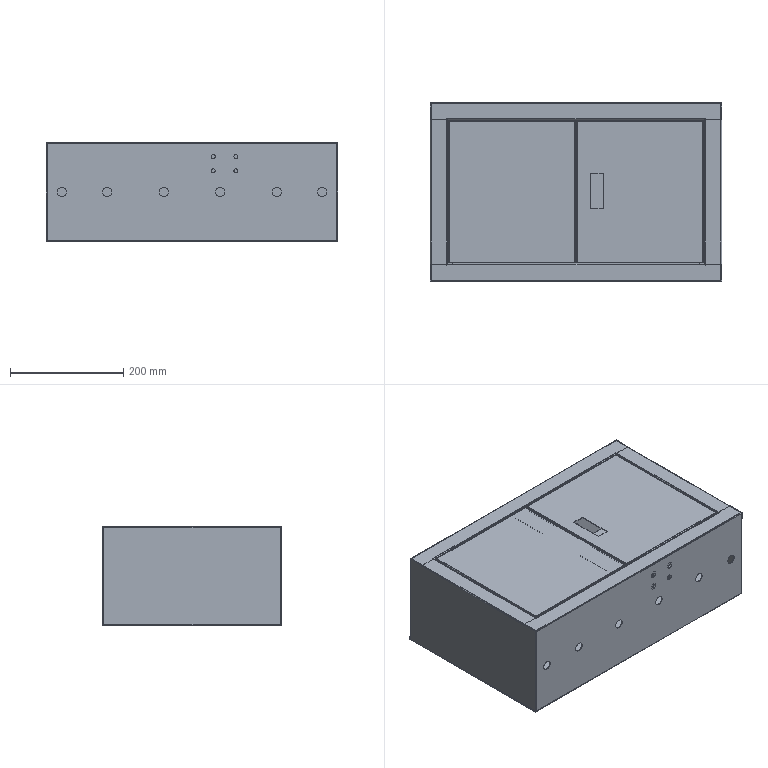Part | 7 solids | 544 faces | box 515 x 315 x 175 mm | volume 1042494 mm3 | plane 394 | cylinder 150 | commonest cylinder face diameters 0.2 x34 3.2 x34 2.5 x16 5.2 x16 10 x14 16 x12